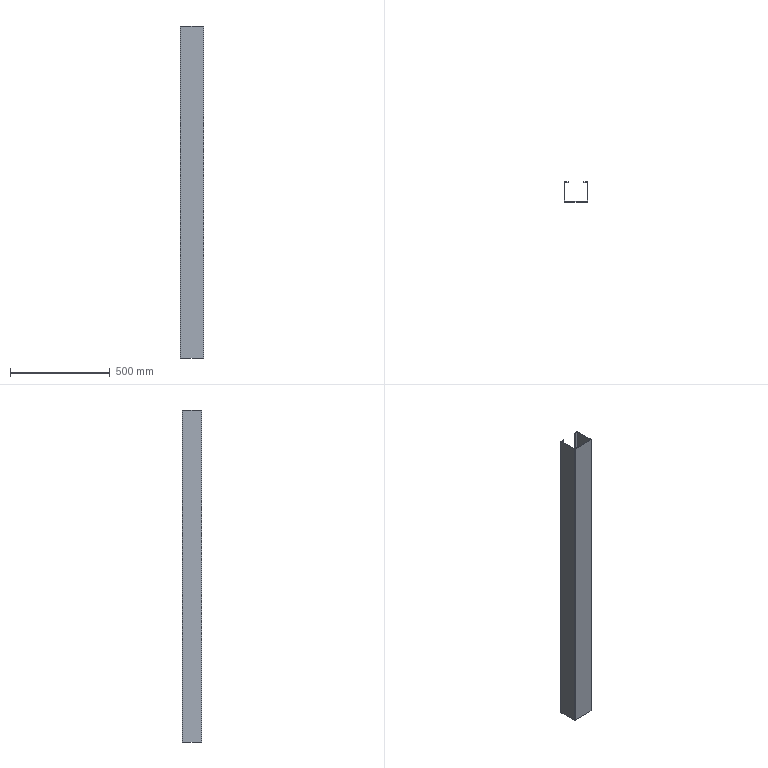Part | STEP file | TS-021-01 | 1 solid | 70 faces | box 120 x 100 x 1668 mm | volume 1716670 mm3 | plane 62 | cylinder 8 | commonest cylinder face diameters 0.4 x4 6.4 x4